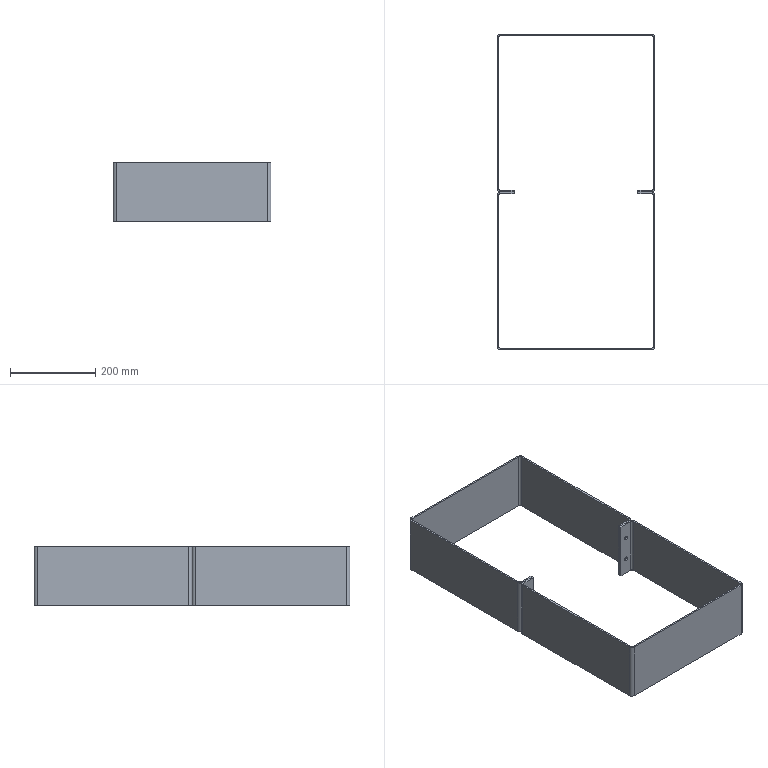Part | SolidWorks | 2 solids | 92 faces | box 370 x 740 x 140 mm | volume 1300830 mm3 | plane 60 | cylinder 32 | commonest cylinder face diameters 10 x16 8 x8 16 x8